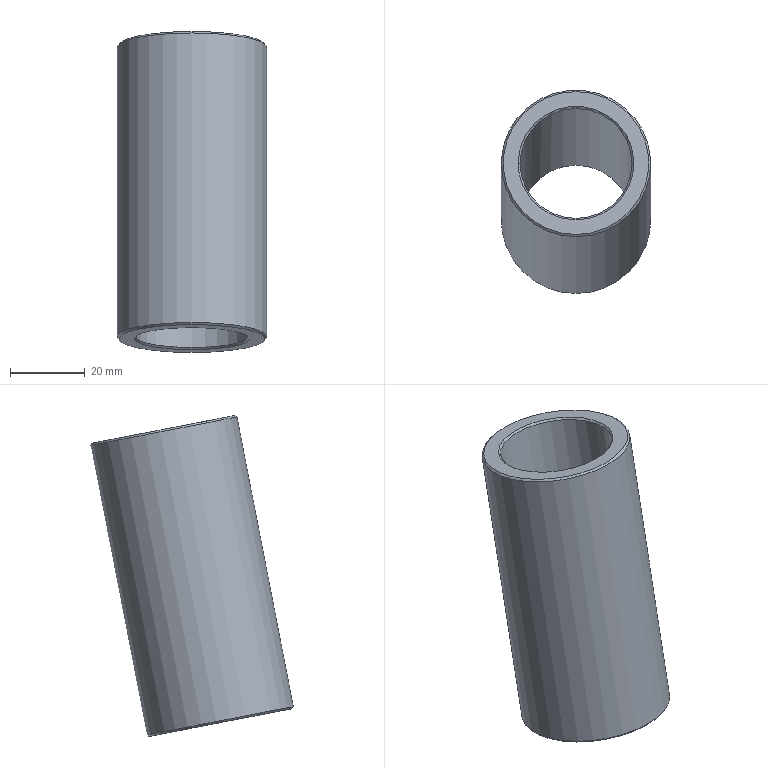Part | STEP file | solid 83 | 1 solid | 8 faces | box 40 x 54.339 x 85.972 mm | volume 43927 mm3 | cone 4 | plane 2 | cylinder 2 | commonest cylinder face diameters 30 x1 40 x1